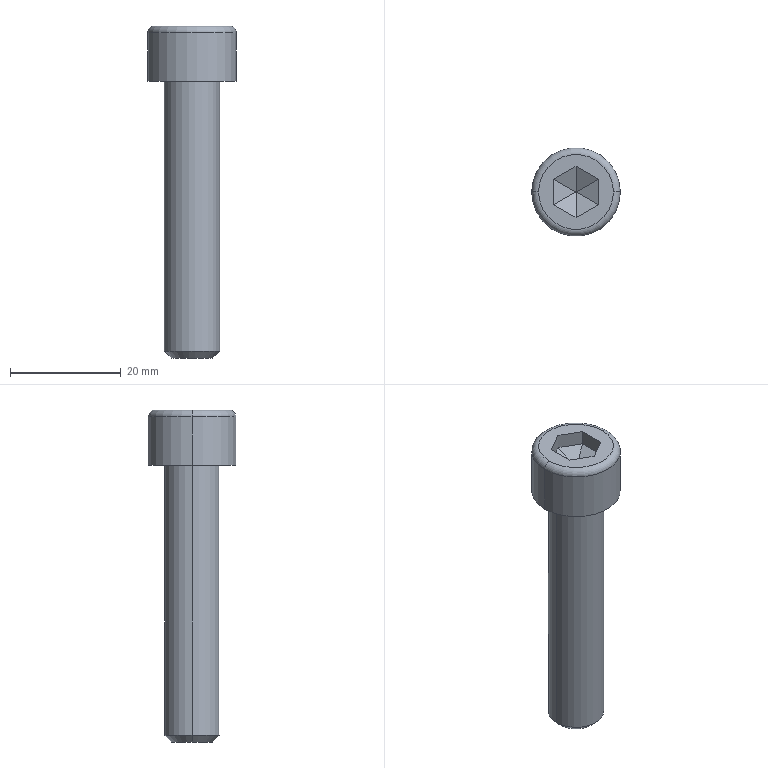Part | SolidWorks | features Chamfer 2, Fillet 2, ICE 2, Extrusion 1, RefAxis 1 | 1 solid | 26 faces | box 16 x 16 x 60 mm | volume 5707 mm3 | plane 16 | torus 4 | cylinder 4 | cone 2 | commonest cylinder face diameters 10 x2 16 x2
STEP:
#1=CARTESIAN_POINT('',(-5.1,0.,0.));
#2=VERTEX_POINT('',#1);
#3=CARTESIAN_POINT('',(5.1,0.,0.));
#4=VERTEX_POINT('',#3);
#5=CARTESIAN_POINT('',(0.,0.,0.));
#6=DIRECTION('',(0.,0.,1.));
#7=DIRECTION('',(1.,0.,0.));
#8=AXIS2_PLACEMENT_3D('',#5,#6,#7);
#9=CIRCLE('',#8,5.1);
#10=EDGE_CURVE('',#2,#4,#9,.T.);
#11=ORIENTED_EDGE('',*,*,#10,.F.);
#12=CARTESIAN_POINT('',(-5.,0.,-0.1));
#13=VERTEX_POINT('',#12);
#14=CARTESIAN_POINT('',(-5.1,0.,-0.1));
#15=DIRECTION('',(0.,1.,0.));
#16=DIRECTION('',(-1.,0.,0.));
#17=AXIS2_PLACEMENT_3D('',#14,#15,#16);
#18=CIRCLE('',#17,0.1);
#19=EDGE_CURVE('',#2,#13,#18,.T.);
#20=ORIENTED_EDGE('',*,*,#19,.T.);
#21=CARTESIAN_POINT('',(5.,0.,-0.1));
#22=VERTEX_POINT('',#21);
#23=CARTESIAN_POINT('',(0.,0.,-0.1));
#24=DIRECTION('',(0.,0.,-1.));
#25=DIRECTION('',(1.,0.,0.));
#26=AXIS2_PLACEMENT_3D('',#23,#24,#25);
#27=CIRCLE('',#26,5.);
#28=EDGE_CURVE('',#22,#13,#27,.T.);
#29=ORIENTED_EDGE('',*,*,#28,.F.);
#30=CARTESIAN_POINT('',(5.1,0.,-0.1));
#31=DIRECTION('',(0.,-1.,0.));
#32=DIRECTION('',(0.,0.,-1.));
#33=AXIS2_PLACEMENT_3D('',#30,#31,#32);
#34=CIRCLE('',#33,0.1);
#35=EDGE_CURVE('',#4,#22,#34,.T.);
#36=ORIENTED_EDGE('',*,*,#35,.F.);
#37=EDGE_LOOP('',(#11,#20,#29,#36));
#38=FACE_OUTER_BOUND('',#37,.T.);
#39=CARTESIAN_POINT('',(0.,0.,-0.1));
#40=DIRECTION('',(0.,0.,1.));
#41=DIRECTION('',(1.,0.,0.));
#42=AXIS2_PLACEMENT_3D('',#39,#40,#41);
#43=TOROIDAL_SURFACE('',#42,5.1,0.1);
#44=ADVANCED_FACE('',(#38),#43,.F.);
#45=CARTESIAN_POINT('',(-8.,0.,8.769));
#46=VERTEX_POINT('',#45);
#47=CARTESIAN_POINT('',(8.,0.,8.769));
#48=VERTEX_POINT('',#47);
#49=CARTESIAN_POINT('',(0.,0.,8.769));
#50=DIRECTION('',(0.,0.,-1.));
#51=DIRECTION('',(1.,0.,0.));
#52=AXIS2_PLACEMENT_3D('',#49,#50,#51);
#53=CIRCLE('',#52,8.);
#54=EDGE_CURVE('',#46,#48,#53,.T.);
#55=ORIENTED_EDGE('',*,*,#54,.F.);
#56=CARTESIAN_POINT('',(-6.769,0.,10.));
#57=VERTEX_POINT('',#56);
#58=CARTESIAN_POINT('',(-6.769,0.,8.769));
#59=DIRECTION('',(0.,1.,0.));
#60=DIRECTION('',(-1.,0.,0.));
#61=AXIS2_PLACEMENT_3D('',#58,#59,#60);
#62=CIRCLE('',#61,1.231);
#63=EDGE_CURVE('',#46,#57,#62,.T.);
#64=ORIENTED_EDGE('',*,*,#63,.T.);
#65=CARTESIAN_POINT('',(6.769,0.,10.));
#66=VERTEX_POINT('',#65);
#67=CARTESIAN_POINT('',(0.,0.,10.));
#68=DIRECTION('',(0.,0.,1.));
#69=DIRECTION('',(1.,0.,0.));
#70=AXIS2_PLACEMENT_3D('',#67,#68,#69);
#71=CIRCLE('',#70,6.769);
#72=EDGE_CURVE('',#66,#57,#71,.T.);
#73=ORIENTED_EDGE('',*,*,#72,.F.);
#74=CARTESIAN_POINT('',(6.769,0.,8.769));
#75=DIRECTION('',(0.,-1.,0.));
#76=DIRECTION('',(0.,0.,-1.));
#77=AXIS2_PLACEMENT_3D('',#74,#75,#76);
#78=CIRCLE('',#77,1.231);
#79=EDGE_CURVE('',#48,#66,#78,.T.);
#80=ORIENTED_EDGE('',*,*,#79,.F.);
#81=EDGE_LOOP('',(#55,#64,#73,#80));
#82=FACE_OUTER_BOUND('',#81,.T.);
#83=CARTESIAN_POINT('',(0.,0.,8.769));
#84=DIRECTION('',(0.,0.,1.));
#85=DIRECTION('',(1.,0.,0.));
#86=AXIS2_PLACEMENT_3D('',#83,#84,#85);
#87=TOROIDAL_SURFACE('',#86,6.769,1.231);
#88=ADVANCED_FACE('',(#82),#87,.T.);
#89=CARTESIAN_POINT('',(-3.75,0.,-50.));
#90=VERTEX_POINT('',#89);
#91=CARTESIAN_POINT('',(3.75,0.,-50.));
#92=VERTEX_POINT('',#91);
#93=CARTESIAN_POINT('',(0.,0.,-50.));
#94=DIRECTION('',(0.,0.,-1.));
#95=DIRECTION('',(-1.,0.,0.));
#96=AXIS2_PLACEMENT_3D('',#93,#94,#95);
#97=CIRCLE('',#96,3.75);
#98=EDGE_CURVE('',#90,#92,#97,.T.);
#99=ORIENTED_EDGE('',*,*,#98,.F.);
#100=CARTESIAN_POINT('',(-5.,0.,-48.75));
#101=VERTEX_POINT('',#100);
#102=CARTESIAN_POINT('',(-3.75,0.,-50.));
#103=DIRECTION('',(-0.7071,0.,0.7071));
#104=VECTOR('',#103,1000.);
#105=LINE('',#102,#104);
#106=EDGE_CURVE('',#90,#101,#105,.T.);
#107=ORIENTED_EDGE('',*,*,#106,.T.);
#108=CARTESIAN_POINT('',(5.,0.,-48.75));
#109=VERTEX_POINT('',#108);
#110=CARTESIAN_POINT('',(0.,0.,-48.75));
#111=DIRECTION('',(0.,0.,1.));
#112=DIRECTION('',(-1.,0.,0.));
#113=AXIS2_PLACEMENT_3D('',#110,#111,#112);
#114=CIRCLE('',#113,5.);
#115=EDGE_CURVE('',#109,#101,#114,.T.);
#116=ORIENTED_EDGE('',*,*,#115,.F.);
#117=CARTESIAN_POINT('',(3.75,0.,-50.));
#118=DIRECTION('',(0.7071,0.,0.7071));
#119=VECTOR('',#118,1000.);
#120=LINE('',#117,#119);
#121=EDGE_CURVE('',#92,#109,#120,.T.);
#122=ORIENTED_EDGE('',*,*,#121,.F.);
#123=EDGE_LOOP('',(#99,#107,#116,#122));
#124=FACE_OUTER_BOUND('',#123,.T.);
#125=CARTESIAN_POINT('',(0.,0.,-50.));
#126=DIRECTION('',(0.,0.,1.));
#127=DIRECTION('',(1.,0.,0.));
#128=AXIS2_PLACEMENT_3D('',#125,#126,#127);
#129=CONICAL_SURFACE('',#128,3.75,0.7854);
#130=ADVANCED_FACE('',(#124),#129,.T.);
#131=ORIENTED_EDGE('',*,*,#115,.T.);
#132=CARTESIAN_POINT('',(-5.,0.,-50.));
#133=DIRECTION('',(0.,0.,1.));
#134=VECTOR('',#133,1000.);
#135=LINE('',#132,#134);
#136=EDGE_CURVE('',#101,#13,#135,.T.);
#137=ORIENTED_EDGE('',*,*,#136,.T.);
#138=CARTESIAN_POINT('',(0.,0.,-0.1));
#139=DIRECTION('',(0.,0.,-1.));
#140=DIRECTION('',(1.,0.,0.));
#141=AXIS2_PLACEMENT_3D('',#138,#139,#140);
#142=CIRCLE('',#141,5.);
#143=EDGE_CURVE('',#13,#22,#142,.T.);
#144=ORIENTED_EDGE('',*,*,#143,.T.);
#145=CARTESIAN_POINT('',(5.,0.,-50.));
#146=DIRECTION('',(0.,0.,1.));
#147=VECTOR('',#146,1000.);
#148=LINE('',#145,#147);
#149=EDGE_CURVE('',#109,#22,#148,.T.);
#150=ORIENTED_EDGE('',*,*,#149,.F.);
#151=EDGE_LOOP('',(#131,#137,#144,#150));
#152=FACE_OUTER_BOUND('',#151,.T.);
#153=CARTESIAN_POINT('',(0.,0.,-50.));
#154=DIRECTION('',(0.,0.,1.));
#155=DIRECTION('',(1.,0.,0.));
#156=AXIS2_PLACEMENT_3D('',#153,#154,#155);
#157=CYLINDRICAL_SURFACE('',#156,5.);
#158=ADVANCED_FACE('',(#152),#157,.T.);
#159=ORIENTED_EDGE('',*,*,#54,.T.);
#160=CARTESIAN_POINT('',(8.,0.,0.));
#161=VERTEX_POINT('',#160);
#162=CARTESIAN_POINT('',(8.,0.,10.));
#163=DIRECTION('',(0.,0.,-1.));
#164=VECTOR('',#163,1000.);
#165=LINE('',#162,#164);
#166=EDGE_CURVE('',#48,#161,#165,.T.);
#167=ORIENTED_EDGE('',*,*,#166,.T.);
#168=CARTESIAN_POINT('',(-8.,0.,0.));
#169=VERTEX_POINT('',#168);
#170=CARTESIAN_POINT('',(0.,0.,0.));
#171=DIRECTION('',(0.,0.,1.));
#172=DIRECTION('',(1.,0.,0.));
#173=AXIS2_PLACEMENT_3D('',#170,#171,#172);
#174=CIRCLE('',#173,8.);
#175=EDGE_CURVE('',#161,#169,#174,.T.);
#176=ORIENTED_EDGE('',*,*,#175,.T.);
#177=CARTESIAN_POINT('',(-8.,0.,10.));
#178=DIRECTION('',(0.,0.,-1.));
#179=VECTOR('',#178,1000.);
#180=LINE('',#177,#179);
#181=EDGE_CURVE('',#46,#169,#180,.T.);
#182=ORIENTED_EDGE('',*,*,#181,.F.);
#183=EDGE_LOOP('',(#159,#167,#176,#182));
#184=FACE_OUTER_BOUND('',#183,.T.);
#185=CARTESIAN_POINT('',(0.,0.,10.));
#186=DIRECTION('',(0.,0.,-1.));
#187=DIRECTION('',(-1.,0.,0.));
#188=AXIS2_PLACEMENT_3D('',#185,#186,#187);
#189=CYLINDRICAL_SURFACE('',#188,8.);
#190=ADVANCED_FACE('',(#184),#189,.T.);
#191=CARTESIAN_POINT('',(0.,0.,0.));
#192=DIRECTION('',(0.,0.,1.));
#193=DIRECTION('',(1.,0.,0.));
#194=AXIS2_PLACEMENT_3D('',#191,#192,#193);
#195=CIRCLE('',#194,5.1);
#196=EDGE_CURVE('',#4,#2,#195,.T.);
#197=ORIENTED_EDGE('',*,*,#196,.T.);
#198=ORIENTED_EDGE('',*,*,#10,.T.);
#199=EDGE_LOOP('',(#197,#198));
#200=FACE_BOUND('',#199,.T.);
#201=CARTESIAN_POINT('',(0.,0.,0.));
#202=DIRECTION('',(0.,0.,1.));
#203=DIRECTION('',(1.,0.,0.));
#204=AXIS2_PLACEMENT_3D('',#201,#202,#203);
#205=CIRCLE('',#204,8.);
#206=EDGE_CURVE('',#169,#161,#205,.T.);
#207=ORIENTED_EDGE('',*,*,#206,.F.);
#208=ORIENTED_EDGE('',*,*,#175,.F.);
#209=EDGE_LOOP('',(#207,#208));
#210=FACE_OUTER_BOUND('',#209,.T.);
#211=CARTESIAN_POINT('',(0.,0.,0.));
#212=DIRECTION('',(0.,0.,1.));
#213=DIRECTION('',(1.,0.,0.));
#214=AXIS2_PLACEMENT_3D('',#211,#212,#213);
#215=PLANE('',#214);
#216=ADVANCED_FACE('',(#200,#210),#215,.F.);
#217=ORIENTED_EDGE('',*,*,#166,.F.);
#218=CARTESIAN_POINT('',(0.,0.,8.769));
#219=DIRECTION('',(0.,0.,-1.));
#220=DIRECTION('',(1.,0.,0.));
#221=AXIS2_PLACEMENT_3D('',#218,#219,#220);
#222=CIRCLE('',#221,8.);
#223=EDGE_CURVE('',#48,#46,#222,.T.);
#224=ORIENTED_EDGE('',*,*,#223,.T.);
#225=ORIENTED_EDGE('',*,*,#181,.T.);
#226=ORIENTED_EDGE('',*,*,#206,.T.);
#227=EDGE_LOOP('',(#217,#224,#225,#226));
#228=FACE_OUTER_BOUND('',#227,.T.);
#229=CARTESIAN_POINT('',(0.,0.,10.));
#230=DIRECTION('',(0.,0.,-1.));
#231=DIRECTION('',(-1.,0.,0.));
#232=AXIS2_PLACEMENT_3D('',#229,#230,#231);
#233=CYLINDRICAL_SURFACE('',#232,8.);
#234=ADVANCED_FACE('',(#228),#233,.T.);
#235=ORIENTED_EDGE('',*,*,#72,.T.);
#236=CARTESIAN_POINT('',(0.,0.,10.));
#237=DIRECTION('',(0.,0.,1.));
#238=DIRECTION('',(1.,0.,0.));
#239=AXIS2_PLACEMENT_3D('',#236,#237,#238);
#240=CIRCLE('',#239,6.769);
#241=EDGE_CURVE('',#57,#66,#240,.T.);
#242=ORIENTED_EDGE('',*,*,#241,.T.);
#243=EDGE_LOOP('',(#235,#242));
#244=FACE_OUTER_BOUND('',#243,.T.);
#245=CARTESIAN_POINT('',(4.,-2.309,10.));
#246=VERTEX_POINT('',#245);
#247=CARTESIAN_POINT('',(4.,2.309,10.));
#248=VERTEX_POINT('',#247);
#249=CARTESIAN_POINT('',(4.,-2.309,10.));
#250=DIRECTION('',(0.,1.,0.));
#251=VECTOR('',#250,1000.);
#252=LINE('',#249,#251);
#253=EDGE_CURVE('',#246,#248,#252,.T.);
#254=ORIENTED_EDGE('',*,*,#253,.F.);
#255=CARTESIAN_POINT('',(0.,-4.619,10.));
#256=VERTEX_POINT('',#255);
#257=CARTESIAN_POINT('',(0.,-4.619,10.));
#258=DIRECTION('',(0.866,0.5,0.));
#259=VECTOR('',#258,1000.);
#260=LINE('',#257,#259);
#261=EDGE_CURVE('',#256,#246,#260,.T.);
#262=ORIENTED_EDGE('',*,*,#261,.F.);
#263=CARTESIAN_POINT('',(-4.,-2.309,10.));
#264=VERTEX_POINT('',#263);
#265=CARTESIAN_POINT('',(-4.,-2.309,10.));
#266=DIRECTION('',(0.866,-0.5,0.));
#267=VECTOR('',#266,1000.);
#268=LINE('',#265,#267);
#269=EDGE_CURVE('',#264,#256,#268,.T.);
#270=ORIENTED_EDGE('',*,*,#269,.F.);
#271=CARTESIAN_POINT('',(-4.,2.309,10.));
#272=VERTEX_POINT('',#271);
#273=CARTESIAN_POINT('',(-4.,2.309,10.));
#274=DIRECTION('',(0.,-1.,0.));
#275=VECTOR('',#274,1000.);
#276=LINE('',#273,#275);
#277=EDGE_CURVE('',#272,#264,#276,.T.);
#278=ORIENTED_EDGE('',*,*,#277,.F.);
#279=CARTESIAN_POINT('',(0.,4.619,10.));
#280=VERTEX_POINT('',#279);
#281=CARTESIAN_POINT('',(0.,4.619,10.));
#282=DIRECTION('',(-0.866,-0.5,0.));
#283=VECTOR('',#282,1000.);
#284=LINE('',#281,#283);
#285=EDGE_CURVE('',#280,#272,#284,.T.);
#286=ORIENTED_EDGE('',*,*,#285,.F.);
#287=CARTESIAN_POINT('',(4.,2.309,10.));
#288=DIRECTION('',(-0.866,0.5,0.));
#289=VECTOR('',#288,1000.);
#290=LINE('',#287,#289);
#291=EDGE_CURVE('',#248,#280,#290,.T.);
#292=ORIENTED_EDGE('',*,*,#291,.F.);
#293=EDGE_LOOP('',(#254,#262,#270,#278,#286,#292));
#294=FACE_BOUND('',#293,.T.);
#295=CARTESIAN_POINT('',(0.,0.,10.));
#296=DIRECTION('',(0.,0.,1.));
#297=DIRECTION('',(1.,0.,0.));
#298=AXIS2_PLACEMENT_3D('',#295,#296,#297);
#299=PLANE('',#298);
#300=ADVANCED_FACE('',(#244,#294),#299,.T.);
#301=CARTESIAN_POINT('',(4.,2.309,7.305));
#302=VERTEX_POINT('',#301);
#303=CARTESIAN_POINT('',(4.,2.309,5.));
#304=DIRECTION('',(0.,0.,1.));
#305=VECTOR('',#304,1000.);
#306=LINE('',#303,#305);
#307=EDGE_CURVE('',#302,#248,#306,.T.);
#308=ORIENTED_EDGE('',*,*,#307,.F.);
#309=CARTESIAN_POINT('',(4.,-2.309,7.305));
#310=VERTEX_POINT('',#309);
#311=CARTESIAN_POINT('',(4.,-2.309,7.305));
#312=DIRECTION('',(0.,-1.,0.));
#313=VECTOR('',#312,1000.);
#314=LINE('',#311,#313);
#315=EDGE_CURVE('',#302,#310,#314,.T.);
#316=ORIENTED_EDGE('',*,*,#315,.T.);
#317=CARTESIAN_POINT('',(4.,-2.309,5.));
#318=DIRECTION('',(0.,0.,1.));
#319=VECTOR('',#318,1000.);
#320=LINE('',#317,#319);
#321=EDGE_CURVE('',#310,#246,#320,.T.);
#322=ORIENTED_EDGE('',*,*,#321,.T.);
#323=ORIENTED_EDGE('',*,*,#253,.T.);
#324=EDGE_LOOP('',(#308,#316,#322,#323));
#325=FACE_OUTER_BOUND('',#324,.T.);
#326=CARTESIAN_POINT('',(4.,-2.309,5.));
#327=DIRECTION('',(1.,0.,0.));
#328=DIRECTION('',(0.,1.,0.));
#329=AXIS2_PLACEMENT_3D('',#326,#327,#328);
#330=PLANE('',#329);
#331=ADVANCED_FACE('',(#325),#330,.F.);
#332=ORIENTED_EDGE('',*,*,#321,.F.);
#333=CARTESIAN_POINT('',(0.,-4.619,7.305));
#334=VERTEX_POINT('',#333);
#335=CARTESIAN_POINT('',(0.,-4.619,7.305));
#336=DIRECTION('',(-0.866,-0.5,0.));
#337=VECTOR('',#336,1000.);
#338=LINE('',#335,#337);
#339=EDGE_CURVE('',#310,#334,#338,.T.);
#340=ORIENTED_EDGE('',*,*,#339,.T.);
#341=CARTESIAN_POINT('',(0.,-4.619,5.));
#342=DIRECTION('',(0.,0.,1.));
#343=VECTOR('',#342,1000.);
#344=LINE('',#341,#343);
#345=EDGE_CURVE('',#334,#256,#344,.T.);
#346=ORIENTED_EDGE('',*,*,#345,.T.);
#347=ORIENTED_EDGE('',*,*,#261,.T.);
#348=EDGE_LOOP('',(#332,#340,#346,#347));
#349=FACE_OUTER_BOUND('',#348,.T.);
#350=CARTESIAN_POINT('',(0.,-4.619,5.));
#351=DIRECTION('',(0.5,-0.866,0.));
#352=DIRECTION('',(0.866,0.5,0.));
#353=AXIS2_PLACEMENT_3D('',#350,#351,#352);
#354=PLANE('',#353);
#355=ADVANCED_FACE('',(#349),#354,.F.);
#356=ORIENTED_EDGE('',*,*,#345,.F.);
#357=CARTESIAN_POINT('',(-4.,-2.309,7.305));
#358=VERTEX_POINT('',#357);
#359=CARTESIAN_POINT('',(-4.,-2.309,7.305));
#360=DIRECTION('',(-0.866,0.5,0.));
#361=VECTOR('',#360,1000.);
#362=LINE('',#359,#361);
#363=EDGE_CURVE('',#334,#358,#362,.T.);
#364=ORIENTED_EDGE('',*,*,#363,.T.);
#365=CARTESIAN_POINT('',(-4.,-2.309,5.));
#366=DIRECTION('',(0.,0.,1.));
#367=VECTOR('',#366,1000.);
#368=LINE('',#365,#367);
#369=EDGE_CURVE('',#358,#264,#368,.T.);
#370=ORIENTED_EDGE('',*,*,#369,.T.);
#371=ORIENTED_EDGE('',*,*,#269,.T.);
#372=EDGE_LOOP('',(#356,#364,#370,#371));
#373=FACE_OUTER_BOUND('',#372,.T.);
#374=CARTESIAN_POINT('',(-4.,-2.309,5.));
#375=DIRECTION('',(-0.5,-0.866,0.));
#376=DIRECTION('',(0.866,-0.5,0.));
#377=AXIS2_PLACEMENT_3D('',#374,#375,#376);
#378=PLANE('',#377);
#379=ADVANCED_FACE('',(#373),#378,.F.);
#380=ORIENTED_EDGE('',*,*,#369,.F.);
#381=CARTESIAN_POINT('',(-4.,2.309,7.305));
#382=VERTEX_POINT('',#381);
#383=CARTESIAN_POINT('',(-4.,2.309,7.305));
#384=DIRECTION('',(0.,1.,0.));
#385=VECTOR('',#384,1000.);
#386=LINE('',#383,#385);
#387=EDGE_CURVE('',#358,#382,#386,.T.);
#388=ORIENTED_EDGE('',*,*,#387,.T.);
#389=CARTESIAN_POINT('',(-4.,2.309,5.));
#390=DIRECTION('',(0.,0.,1.));
#391=VECTOR('',#390,1000.);
#392=LINE('',#389,#391);
#393=EDGE_CURVE('',#382,#272,#392,.T.);
#394=ORIENTED_EDGE('',*,*,#393,.T.);
#395=ORIENTED_EDGE('',*,*,#277,.T.);
#396=EDGE_LOOP('',(#380,#388,#394,#395));
#397=FACE_OUTER_BOUND('',#396,.T.);
#398=CARTESIAN_POINT('',(-4.,2.309,5.));
#399=DIRECTION('',(-1.,0.,0.));
#400=DIRECTION('',(0.,0.,1.));
#401=AXIS2_PLACEMENT_3D('',#398,#399,#400);
#402=PLANE('',#401);
#403=ADVANCED_FACE('',(#397),#402,.F.);
#404=ORIENTED_EDGE('',*,*,#393,.F.);
#405=CARTESIAN_POINT('',(0.,4.619,7.305));
#406=VERTEX_POINT('',#405);
#407=CARTESIAN_POINT('',(0.,4.619,7.305));
#408=DIRECTION('',(0.866,0.5,0.));
#409=VECTOR('',#408,1000.);
#410=LINE('',#407,#409);
#411=EDGE_CURVE('',#382,#406,#410,.T.);
#412=ORIENTED_EDGE('',*,*,#411,.T.);
#413=CARTESIAN_POINT('',(0.,4.619,5.));
#414=DIRECTION('',(0.,0.,1.));
#415=VECTOR('',#414,1000.);
#416=LINE('',#413,#415);
#417=EDGE_CURVE('',#406,#280,#416,.T.);
#418=ORIENTED_EDGE('',*,*,#417,.T.);
#419=ORIENTED_EDGE('',*,*,#285,.T.);
#420=EDGE_LOOP('',(#404,#412,#418,#419));
#421=FACE_OUTER_BOUND('',#420,.T.);
#422=CARTESIAN_POINT('',(0.,4.619,5.));
#423=DIRECTION('',(-0.5,0.866,0.));
#424=DIRECTION('',(-0.866,-0.5,0.));
#425=AXIS2_PLACEMENT_3D('',#422,#423,#424);
#426=PLANE('',#425);
#427=ADVANCED_FACE('',(#421),#426,.F.);
#428=ORIENTED_EDGE('',*,*,#417,.F.);
#429=CARTESIAN_POINT('',(4.,2.309,7.305));
#430=DIRECTION('',(0.866,-0.5,0.));
#431=VECTOR('',#430,1000.);
#432=LINE('',#429,#431);
#433=EDGE_CURVE('',#406,#302,#432,.T.);
#434=ORIENTED_EDGE('',*,*,#433,.T.);
#435=ORIENTED_EDGE('',*,*,#307,.T.);
#436=ORIENTED_EDGE('',*,*,#291,.T.);
#437=EDGE_LOOP('',(#428,#434,#435,#436));
#438=FACE_OUTER_BOUND('',#437,.T.);
#439=CARTESIAN_POINT('',(4.,2.309,5.));
#440=DIRECTION('',(0.5,0.866,0.));
#441=DIRECTION('',(-0.866,0.5,0.));
#442=AXIS2_PLACEMENT_3D('',#439,#440,#441);
#443=PLANE('',#442);
#444=ADVANCED_FACE('',(#438),#443,.F.);
#445=CARTESIAN_POINT('',(0.,0.007851,5.));
#446=VERTEX_POINT('',#445);
#447=CARTESIAN_POINT('',(-0.006799,0.003926,5.));
#448=VERTEX_POINT('',#447);
#449=CARTESIAN_POINT('',(-0.0034,0.005888,5.));
#450=DIRECTION('',(-0.866,-0.5,0.));
#451=VECTOR('',#450,1000.);
#452=LINE('',#449,#451);
#453=EDGE_CURVE('',#446,#448,#452,.T.);
#454=ORIENTED_EDGE('',*,*,#453,.T.);
#455=CARTESIAN_POINT('',(-0.006799,-0.003926,5.));
#456=VERTEX_POINT('',#455);
#457=CARTESIAN_POINT('',(-0.006799,0.,5.));
#458=DIRECTION('',(0.,-1.,0.));
#459=VECTOR('',#458,1000.);
#460=LINE('',#457,#459);
#461=EDGE_CURVE('',#448,#456,#460,.T.);
#462=ORIENTED_EDGE('',*,*,#461,.T.);
#463=CARTESIAN_POINT('',(0.,-0.007851,5.));
#464=VERTEX_POINT('',#463);
#465=CARTESIAN_POINT('',(-0.0034,-0.005888,5.));
#466=DIRECTION('',(0.866,-0.5,0.));
#467=VECTOR('',#466,1000.);
#468=LINE('',#465,#467);
#469=EDGE_CURVE('',#456,#464,#468,.T.);
#470=ORIENTED_EDGE('',*,*,#469,.T.);
#471=CARTESIAN_POINT('',(0.006799,-0.003926,5.));
#472=VERTEX_POINT('',#471);
#473=CARTESIAN_POINT('',(0.0034,-0.005888,5.));
#474=DIRECTION('',(0.866,0.5,0.));
#475=VECTOR('',#474,1000.);
#476=LINE('',#473,#475);
#477=EDGE_CURVE('',#464,#472,#476,.T.);
#478=ORIENTED_EDGE('',*,*,#477,.T.);
#479=CARTESIAN_POINT('',(0.006799,0.003926,5.));
#480=VERTEX_POINT('',#479);
#481=CARTESIAN_POINT('',(0.006799,0.,5.));
#482=DIRECTION('',(0.,1.,0.));
#483=VECTOR('',#482,1000.);
#484=LINE('',#481,#483);
#485=EDGE_CURVE('',#472,#480,#484,.T.);
#486=ORIENTED_EDGE('',*,*,#485,.T.);
#487=CARTESIAN_POINT('',(0.0034,0.005888,5.));
#488=DIRECTION('',(-0.866,0.5,0.));
#489=VECTOR('',#488,1000.);
#490=LINE('',#487,#489);
#491=EDGE_CURVE('',#480,#446,#490,.T.);
#492=ORIENTED_EDGE('',*,*,#491,.T.);
#493=EDGE_LOOP('',(#454,#462,#470,#478,#486,#492));
#494=FACE_OUTER_BOUND('',#493,.T.);
#495=CARTESIAN_POINT('',(0.,0.,5.));
#496=DIRECTION('',(0.,0.,1.));
#497=DIRECTION('',(1.,0.,0.));
#498=AXIS2_PLACEMENT_3D('',#495,#496,#497);
#499=PLANE('',#498);
#500=ADVANCED_FACE('',(#494),#499,.T.);
#501=ORIENTED_EDGE('',*,*,#136,.F.);
#502=CARTESIAN_POINT('',(0.,0.,-48.75));
#503=DIRECTION('',(0.,0.,1.));
#504=DIRECTION('',(-1.,0.,0.));
#505=AXIS2_PLACEMENT_3D('',#502,#503,#504);
#506=CIRCLE('',#505,5.);
#507=EDGE_CURVE('',#101,#109,#506,.T.);
#508=ORIENTED_EDGE('',*,*,#507,.T.);
#509=ORIENTED_EDGE('',*,*,#149,.T.);
#510=ORIENTED_EDGE('',*,*,#28,.T.);
#511=EDGE_LOOP('',(#501,#508,#509,#510));
#512=FACE_OUTER_BOUND('',#511,.T.);
#513=CARTESIAN_POINT('',(0.,0.,-50.));
#514=DIRECTION('',(0.,0.,1.));
#515=DIRECTION('',(1.,0.,0.));
#516=AXIS2_PLACEMENT_3D('',#513,#514,#515);
#517=CYLINDRICAL_SURFACE('',#516,5.);
#518=ADVANCED_FACE('',(#512),#517,.T.);
#519=CARTESIAN_POINT('',(0.,0.,-50.));
#520=DIRECTION('',(0.,0.,-1.));
#521=DIRECTION('',(-1.,0.,0.));
#522=AXIS2_PLACEMENT_3D('',#519,#520,#521);
#523=CIRCLE('',#522,3.75);
#524=EDGE_CURVE('',#92,#90,#523,.T.);
#525=ORIENTED_EDGE('',*,*,#524,.T.);
#526=ORIENTED_EDGE('',*,*,#98,.T.);
#527=EDGE_LOOP('',(#525,#526));
#528=FACE_OUTER_BOUND('',#527,.T.);
#529=CARTESIAN_POINT('',(0.,0.,-50.));
#530=DIRECTION('',(0.,0.,-1.));
#531=DIRECTION('',(-1.,0.,0.));
#532=AXIS2_PLACEMENT_3D('',#529,#530,#531);
#533=PLANE('',#532);
#534=ADVANCED_FACE('',(#528),#533,.T.);
#535=ORIENTED_EDGE('',*,*,#106,.F.);
#536=ORIENTED_EDGE('',*,*,#524,.F.);
#537=ORIENTED_EDGE('',*,*,#121,.T.);
#538=ORIENTED_EDGE('',*,*,#507,.F.);
#539=EDGE_LOOP('',(#535,#536,#537,#538));
#540=FACE_OUTER_BOUND('',#539,.T.);
#541=CARTESIAN_POINT('',(0.,0.,-50.));
#542=DIRECTION('',(0.,0.,1.));
#543=DIRECTION('',(1.,0.,0.));
#544=AXIS2_PLACEMENT_3D('',#541,#542,#543);
#545=CONICAL_SURFACE('',#544,3.75,0.7854);
#546=ADVANCED_FACE('',(#540),#545,.T.);
#547=ORIENTED_EDGE('',*,*,#63,.F.);
#548=ORIENTED_EDGE('',*,*,#223,.F.);
#549=ORIENTED_EDGE('',*,*,#79,.T.);
#550=ORIENTED_EDGE('',*,*,#241,.F.);
#551=EDGE_LOOP('',(#547,#548,#549,#550));
#552=FACE_OUTER_BOUND('',#551,.T.);
#553=CARTESIAN_POINT('',(0.,0.,8.769));
#554=DIRECTION('',(0.,0.,1.));
#555=DIRECTION('',(1.,0.,0.));
#556=AXIS2_PLACEMENT_3D('',#553,#554,#555);
#557=TOROIDAL_SURFACE('',#556,6.769,1.231);
#558=ADVANCED_FACE('',(#552),#557,.T.);
#559=CARTESIAN_POINT('',(0.005439,-0.00314,4.999));
#560=DIRECTION('',(-0.7746,0.4472,-0.4472));
#561=VECTOR('',#560,1000.);
#562=LINE('',#559,#561);
#563=EDGE_CURVE('',#310,#472,#562,.T.);
#564=ORIENTED_EDGE('',*,*,#563,.F.);
#565=ORIENTED_EDGE('',*,*,#315,.F.);
#566=CARTESIAN_POINT('',(0.005439,0.00314,4.999));
#567=DIRECTION('',(0.7746,0.4472,0.4472));
#568=VECTOR('',#567,1000.);
#569=LINE('',#566,#568);
#570=EDGE_CURVE('',#480,#302,#569,.T.);
#571=ORIENTED_EDGE('',*,*,#570,.F.);
#572=ORIENTED_EDGE('',*,*,#485,.F.);
#573=EDGE_LOOP('',(#564,#565,#571,#572));
#574=FACE_OUTER_BOUND('',#573,.T.);
#575=CARTESIAN_POINT('',(0.006799,0.,5.));
#576=DIRECTION('',(0.5,0.,-0.866));
#577=DIRECTION('',(0.,1.,0.));
#578=AXIS2_PLACEMENT_3D('',#575,#576,#577);
#579=PLANE('',#578);
#580=ADVANCED_FACE('',(#574),#579,.F.);
#581=ORIENTED_EDGE('',*,*,#570,.T.);
#582=ORIENTED_EDGE('',*,*,#433,.F.);
#583=CARTESIAN_POINT('',(0.,0.006281,4.999));
#584=DIRECTION('',(0.,0.8944,0.4472));
#585=VECTOR('',#584,1000.);
#586=LINE('',#583,#585);
#587=EDGE_CURVE('',#446,#406,#586,.T.);
#588=ORIENTED_EDGE('',*,*,#587,.F.);
#589=ORIENTED_EDGE('',*,*,#491,.F.);
#590=EDGE_LOOP('',(#581,#582,#588,#589));
#591=FACE_OUTER_BOUND('',#590,.T.);
#592=CARTESIAN_POINT('',(0.0034,0.005888,5.));
#593=DIRECTION('',(0.25,0.433,-0.866));
#594=DIRECTION('',(-0.866,0.5,0.));
#595=AXIS2_PLACEMENT_3D('',#592,#593,#594);
#596=PLANE('',#595);
#597=ADVANCED_FACE('',(#591),#596,.F.);
#598=ORIENTED_EDGE('',*,*,#563,.T.);
#599=ORIENTED_EDGE('',*,*,#477,.F.);
#600=CARTESIAN_POINT('',(0.,-0.006281,4.999));
#601=DIRECTION('',(0.,0.8944,-0.4472));
#602=VECTOR('',#601,1000.);
#603=LINE('',#600,#602);
#604=EDGE_CURVE('',#334,#464,#603,.T.);
#605=ORIENTED_EDGE('',*,*,#604,.F.);
#606=ORIENTED_EDGE('',*,*,#339,.F.);
#607=EDGE_LOOP('',(#598,#599,#605,#606));
#608=FACE_OUTER_BOUND('',#607,.T.);
#609=CARTESIAN_POINT('',(0.0034,-0.005888,5.));
#610=DIRECTION('',(0.25,-0.433,-0.866));
#611=DIRECTION('',(0.866,0.5,0.));
#612=AXIS2_PLACEMENT_3D('',#609,#610,#611);
#613=PLANE('',#612);
#614=ADVANCED_FACE('',(#608),#613,.F.);
#615=ORIENTED_EDGE('',*,*,#587,.T.);
#616=ORIENTED_EDGE('',*,*,#411,.F.);
#617=CARTESIAN_POINT('',(-0.005439,0.00314,4.999));
#618=DIRECTION('',(-0.7746,0.4472,0.4472));
#619=VECTOR('',#618,1000.);
#620=LINE('',#617,#619);
#621=EDGE_CURVE('',#448,#382,#620,.T.);
#622=ORIENTED_EDGE('',*,*,#621,.F.);
#623=ORIENTED_EDGE('',*,*,#453,.F.);
#624=EDGE_LOOP('',(#615,#616,#622,#623));
#625=FACE_OUTER_BOUND('',#624,.T.);
#626=CARTESIAN_POINT('',(-0.0034,0.005888,5.));
#627=DIRECTION('',(-0.25,0.433,-0.866));
#628=DIRECTION('',(-0.866,-0.5,0.));
#629=AXIS2_PLACEMENT_3D('',#626,#627,#628);
#630=PLANE('',#629);
#631=ADVANCED_FACE('',(#625),#630,.F.);
#632=ORIENTED_EDGE('',*,*,#604,.T.);
#633=ORIENTED_EDGE('',*,*,#469,.F.);
#634=CARTESIAN_POINT('',(-0.005439,-0.00314,4.999));
#635=DIRECTION('',(0.7746,0.4472,-0.4472));
#636=VECTOR('',#635,1000.);
#637=LINE('',#634,#636);
#638=EDGE_CURVE('',#358,#456,#637,.T.);
#639=ORIENTED_EDGE('',*,*,#638,.F.);
#640=ORIENTED_EDGE('',*,*,#363,.F.);
#641=EDGE_LOOP('',(#632,#633,#639,#640));
#642=FACE_OUTER_BOUND('',#641,.T.);
#643=CARTESIAN_POINT('',(-0.0034,-0.005888,5.));
#644=DIRECTION('',(-0.25,-0.433,-0.866));
#645=DIRECTION('',(0.866,-0.5,0.));
#646=AXIS2_PLACEMENT_3D('',#643,#644,#645);
#647=PLANE('',#646);
#648=ADVANCED_FACE('',(#642),#647,.F.);
#649=ORIENTED_EDGE('',*,*,#621,.T.);
#650=ORIENTED_EDGE('',*,*,#387,.F.);
#651=ORIENTED_EDGE('',*,*,#638,.T.);
#652=ORIENTED_EDGE('',*,*,#461,.F.);
#653=EDGE_LOOP('',(#649,#650,#651,#652));
#654=FACE_OUTER_BOUND('',#653,.T.);
#655=CARTESIAN_POINT('',(-0.006799,0.,5.));
#656=DIRECTION('',(-0.5,0.,-0.866));
#657=DIRECTION('',(0.,-1.,0.));
#658=AXIS2_PLACEMENT_3D('',#655,#656,#657);
#659=PLANE('',#658);
#660=ADVANCED_FACE('',(#654),#659,.F.);
#661=ORIENTED_EDGE('',*,*,#19,.F.);
#662=ORIENTED_EDGE('',*,*,#196,.F.);
#663=ORIENTED_EDGE('',*,*,#35,.T.);
#664=ORIENTED_EDGE('',*,*,#143,.F.);
#665=EDGE_LOOP('',(#661,#662,#663,#664));
#666=FACE_OUTER_BOUND('',#665,.T.);
#667=CARTESIAN_POINT('',(0.,0.,-0.1));
#668=DIRECTION('',(0.,0.,1.));
#669=DIRECTION('',(1.,0.,0.));
#670=AXIS2_PLACEMENT_3D('',#667,#668,#669);
#671=TOROIDAL_SURFACE('',#670,5.1,0.1);
#672=ADVANCED_FACE('',(#666),#671,.F.);
#673=CLOSED_SHELL('',(#44,#88,#130,#158,#190,#216,#234,#300,#331,#355,#379,#403,#427,#444,#500,#518,#534,#546,#558,#580,#597,#614,#631,#648,#660,#672));
#674=MANIFOLD_SOLID_BREP('',#673);
#675=CARTESIAN_POINT('',(0.,0.,0.));
#676=DIRECTION('',(0.,0.,1.));
#677=DIRECTION('',(1.,0.,0.));
#678=AXIS2_PLACEMENT_3D('',#675,#676,#677);
#679=(LENGTH_UNIT()NAMED_UNIT(*)SI_UNIT(.MILLI.,.METRE.));
#680=UNCERTAINTY_MEASURE_WITH_UNIT(LENGTH_MEASURE(0.00001),#679,'','');
#681=(NAMED_UNIT(*)PLANE_ANGLE_UNIT()SI_UNIT($,.RADIAN.));
#682=(NAMED_UNIT(*)SI_UNIT($,.STERADIAN.)SOLID_ANGLE_UNIT());
#683=(GEOMETRIC_REPRESENTATION_CONTEXT(3)GLOBAL_UNCERTAINTY_ASSIGNED_CONTEXT((#680))GLOBAL_UNIT_ASSIGNED_CONTEXT((#679,#681,#682))REPRESENTATION_CONTEXT('',''));
#684=ADVANCED_BREP_SHAPE_REPRESENTATION('',(#674,#678),#683);